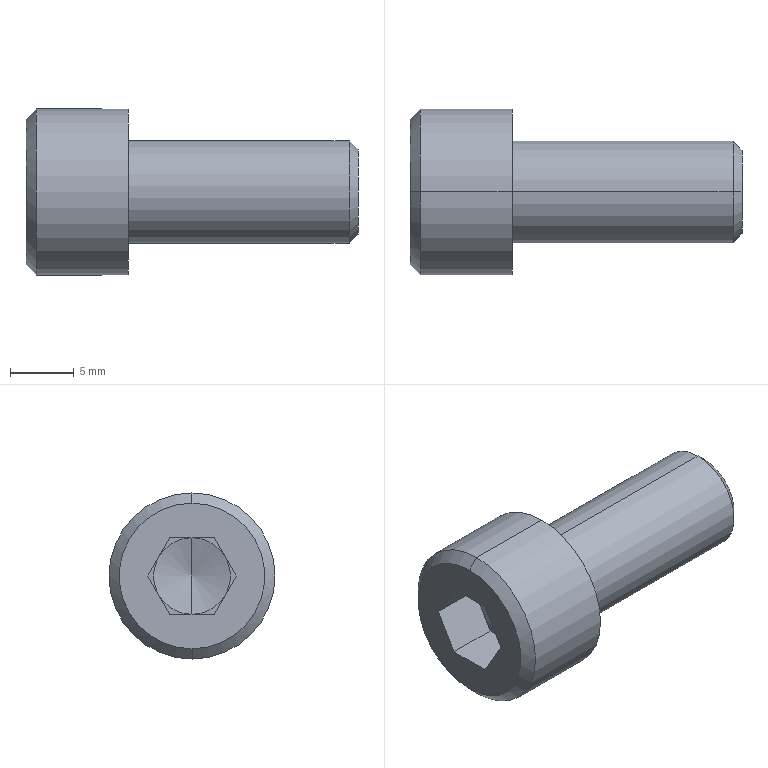Part | STEP file | 0245_310_SCB8-18 | 1 solid | 25 faces | box 26 x 13 x 13 mm | volume 1816 mm3 | plane 15 | cone 6 | cylinder 4 | commonest cylinder face diameters 8 x2 13 x2